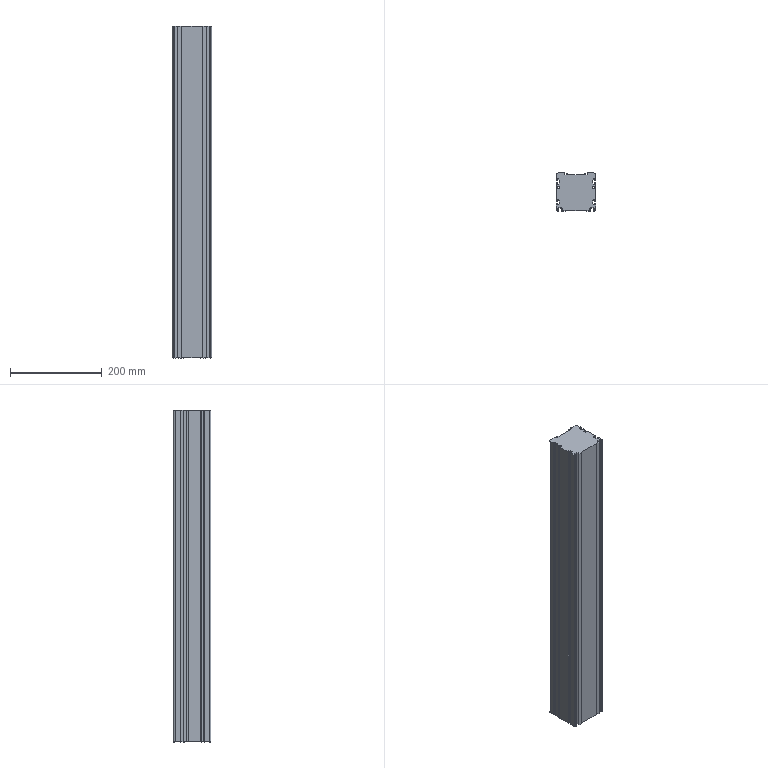Part | STEP file | FFH85-PL-011^FFH85-PL-M75-B3-01_three-axis module | 1 solid | 230 faces | box 85 x 81.5 x 722 mm | volume 4571503 mm3 | plane 118 | cylinder 101 | spline 11 | commonest cylinder face diameters 1 x75 0.6 x16 0.9 x6 4 x2 8 x2